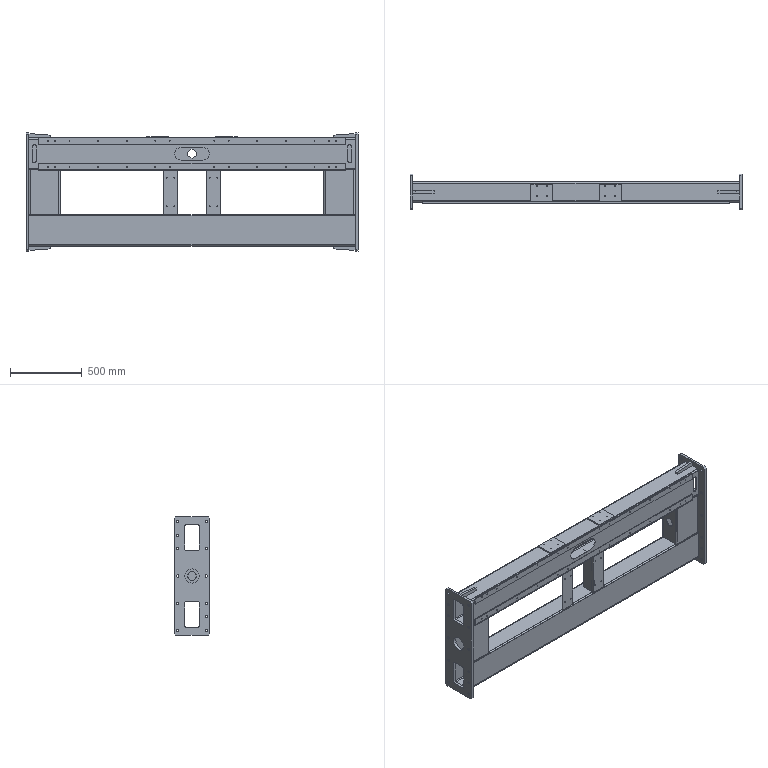Part | SolidWorks | features ICE 14, HoleWzd 6, WeldMemberFeat 3, Chamfer 2, 3DProfileFeature 1, Cut 1, WeldCornerFeat 1, WeldmentFeature 1 | 16 solids | 478 faces | box 2320 x 250 x 830 mm | volume 26047489 mm3 | cylinder 324 | plane 154 | commonest cylinder face diameters 6.8 x128 16.5 x40 5 x36 8.5 x32 20 x32 10 x16